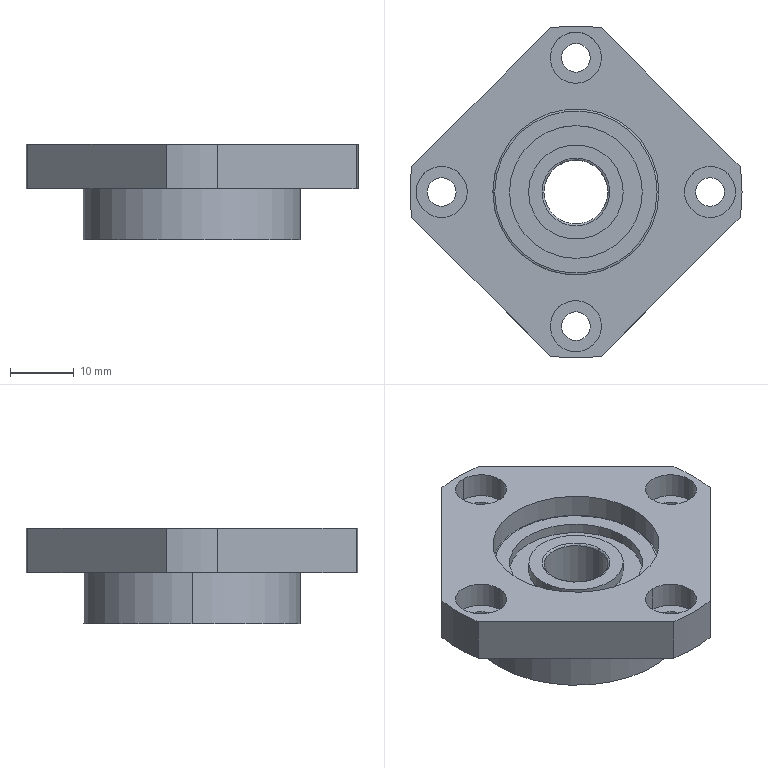Part | SolidWorks | features BaseBody 1 | 1 solid | 62 faces | box 52 x 52 x 15 mm | volume 13321 mm3 | cylinder 37 | plane 17 | spline 8 | commonest cylinder face diameters 4.5 x8 8 x8 52 x5 14.8 x4 20.8 x4 26 x4